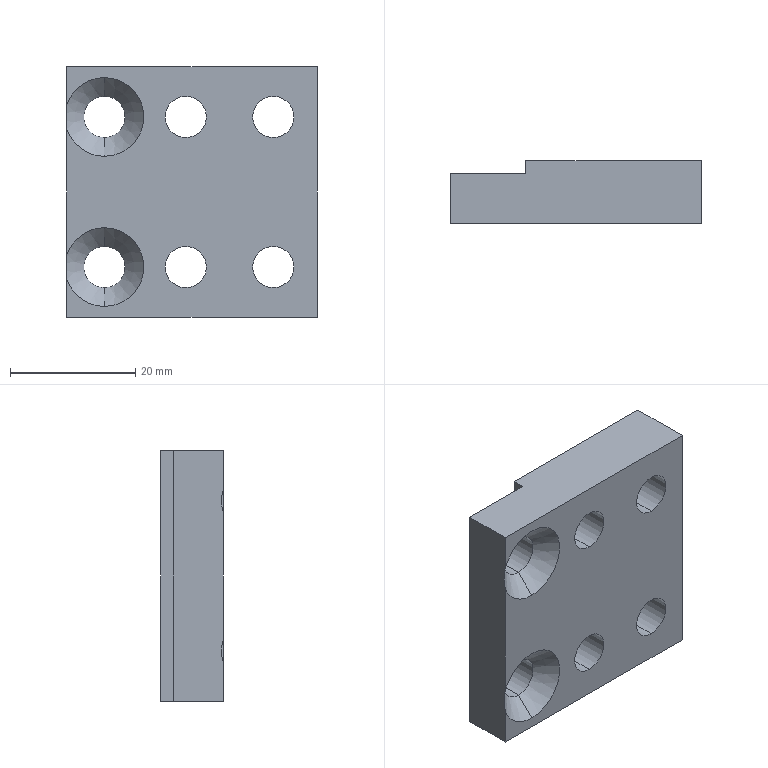Part | STEP file | 1 solid | 32 faces | box 40 x 10 x 40 mm | volume 12395 mm3 | cone 12 | cylinder 12 | plane 8 | commonest cylinder face diameters 6.6 x12